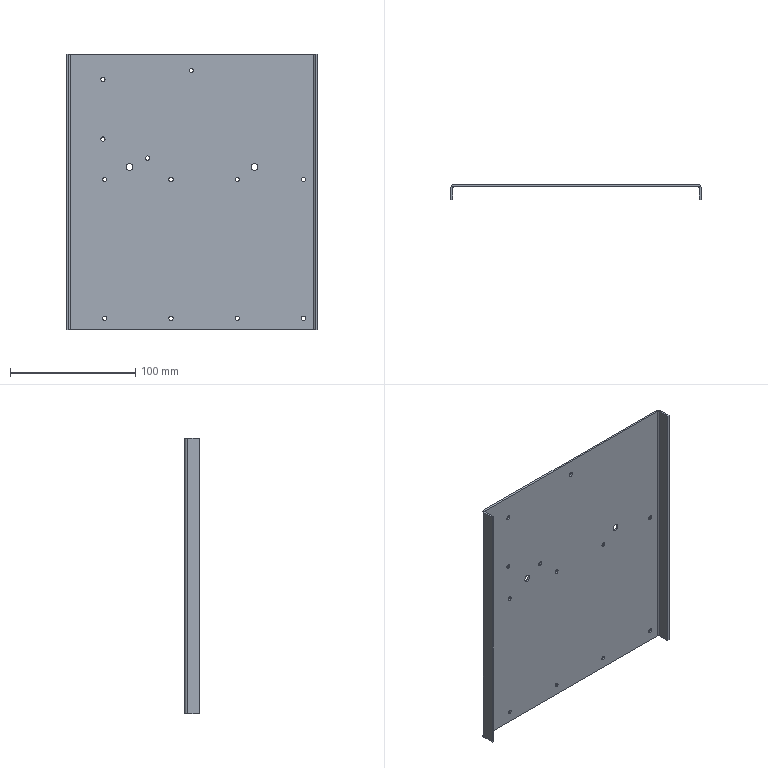Part | NX | features BREP 1 | 1 solid | 28 faces | box 200 x 12 x 220 mm | volume 72200 mm3 | cylinder 18 | plane 10 | commonest cylinder face diameters 3.4 x12 2 x2 5 x2 5.5 x2
STEP:
#1=CARTESIAN_POINT('',(34.5,12.,10.));
#2=VERTEX_POINT('',#1);
#3=CARTESIAN_POINT('',(36.2,12.,10.));
#4=DIRECTION('',(0.,1.,0.));
#5=DIRECTION('',(-1.,0.,0.));
#6=AXIS2_PLACEMENT_3D('',#3,#4,#5);
#7=CIRCLE('',#6,1.7);
#8=EDGE_CURVE('',#2,#2,#7,.T.);
#9=ORIENTED_EDGE('',*,*,#8,.T.);
#10=EDGE_LOOP('',(#9));
#11=FACE_BOUND('',#10,.T.);
#12=CARTESIAN_POINT('',(34.5,10.5,10.));
#13=VERTEX_POINT('',#12);
#14=CARTESIAN_POINT('',(36.2,10.5,10.));
#15=DIRECTION('',(0.,1.,0.));
#16=DIRECTION('',(-1.,0.,0.));
#17=AXIS2_PLACEMENT_3D('',#14,#15,#16);
#18=CIRCLE('',#17,1.7);
#19=EDGE_CURVE('',#13,#13,#18,.T.);
#20=ORIENTED_EDGE('',*,*,#19,.F.);
#21=EDGE_LOOP('',(#20));
#22=FACE_BOUND('',#21,.T.);
#23=CARTESIAN_POINT('',(36.2,2.,10.));
#24=DIRECTION('',(0.,1.,0.));
#25=DIRECTION('',(-1.,0.,0.));
#26=AXIS2_PLACEMENT_3D('',#23,#24,#25);
#27=CYLINDRICAL_SURFACE('',#26,1.7);
#28=ADVANCED_FACE('',(#11,#22),#27,.F.);
#29=CARTESIAN_POINT('',(34.5,12.,-101.));
#30=VERTEX_POINT('',#29);
#31=CARTESIAN_POINT('',(36.2,12.,-101.));
#32=DIRECTION('',(0.,1.,0.));
#33=DIRECTION('',(-1.,0.,0.));
#34=AXIS2_PLACEMENT_3D('',#31,#32,#33);
#35=CIRCLE('',#34,1.7);
#36=EDGE_CURVE('',#30,#30,#35,.T.);
#37=ORIENTED_EDGE('',*,*,#36,.T.);
#38=EDGE_LOOP('',(#37));
#39=FACE_BOUND('',#38,.T.);
#40=CARTESIAN_POINT('',(34.5,10.5,-101.));
#41=VERTEX_POINT('',#40);
#42=CARTESIAN_POINT('',(36.2,10.5,-101.));
#43=DIRECTION('',(0.,1.,0.));
#44=DIRECTION('',(-1.,0.,0.));
#45=AXIS2_PLACEMENT_3D('',#42,#43,#44);
#46=CIRCLE('',#45,1.7);
#47=EDGE_CURVE('',#41,#41,#46,.T.);
#48=ORIENTED_EDGE('',*,*,#47,.F.);
#49=EDGE_LOOP('',(#48));
#50=FACE_BOUND('',#49,.T.);
#51=CARTESIAN_POINT('',(36.2,2.,-101.));
#52=DIRECTION('',(0.,1.,0.));
#53=DIRECTION('',(-1.,0.,0.));
#54=AXIS2_PLACEMENT_3D('',#51,#52,#53);
#55=CYLINDRICAL_SURFACE('',#54,1.7);
#56=ADVANCED_FACE('',(#39,#50),#55,.F.);
#57=CARTESIAN_POINT('',(-72.95,12.,42.321));
#58=VERTEX_POINT('',#57);
#59=CARTESIAN_POINT('',(-71.25,12.,42.321));
#60=DIRECTION('',(0.,1.,0.));
#61=DIRECTION('',(-1.,0.,0.));
#62=AXIS2_PLACEMENT_3D('',#59,#60,#61);
#63=CIRCLE('',#62,1.7);
#64=EDGE_CURVE('',#58,#58,#63,.T.);
#65=ORIENTED_EDGE('',*,*,#64,.T.);
#66=EDGE_LOOP('',(#65));
#67=FACE_BOUND('',#66,.T.);
#68=CARTESIAN_POINT('',(-72.95,10.5,42.321));
#69=VERTEX_POINT('',#68);
#70=CARTESIAN_POINT('',(-71.25,10.5,42.321));
#71=DIRECTION('',(0.,1.,0.));
#72=DIRECTION('',(-1.,0.,0.));
#73=AXIS2_PLACEMENT_3D('',#70,#71,#72);
#74=CIRCLE('',#73,1.7);
#75=EDGE_CURVE('',#69,#69,#74,.T.);
#76=ORIENTED_EDGE('',*,*,#75,.F.);
#77=EDGE_LOOP('',(#76));
#78=FACE_BOUND('',#77,.T.);
#79=CARTESIAN_POINT('',(-71.25,2.,42.321));
#80=DIRECTION('',(0.,1.,0.));
#81=DIRECTION('',(-1.,0.,0.));
#82=AXIS2_PLACEMENT_3D('',#79,#80,#81);
#83=CYLINDRICAL_SURFACE('',#82,1.7);
#84=ADVANCED_FACE('',(#67,#78),#83,.F.);
#85=CARTESIAN_POINT('',(-37.2,12.,27.146));
#86=VERTEX_POINT('',#85);
#87=CARTESIAN_POINT('',(-35.5,12.,27.146));
#88=DIRECTION('',(0.,1.,0.));
#89=DIRECTION('',(-1.,0.,0.));
#90=AXIS2_PLACEMENT_3D('',#87,#88,#89);
#91=CIRCLE('',#90,1.7);
#92=EDGE_CURVE('',#86,#86,#91,.T.);
#93=ORIENTED_EDGE('',*,*,#92,.T.);
#94=EDGE_LOOP('',(#93));
#95=FACE_BOUND('',#94,.T.);
#96=CARTESIAN_POINT('',(-37.2,10.5,27.146));
#97=VERTEX_POINT('',#96);
#98=CARTESIAN_POINT('',(-35.5,10.5,27.146));
#99=DIRECTION('',(0.,1.,0.));
#100=DIRECTION('',(-1.,0.,0.));
#101=AXIS2_PLACEMENT_3D('',#98,#99,#100);
#102=CIRCLE('',#101,1.7);
#103=EDGE_CURVE('',#97,#97,#102,.T.);
#104=ORIENTED_EDGE('',*,*,#103,.F.);
#105=EDGE_LOOP('',(#104));
#106=FACE_BOUND('',#105,.T.);
#107=CARTESIAN_POINT('',(-35.5,2.,27.146));
#108=DIRECTION('',(0.,1.,0.));
#109=DIRECTION('',(-1.,0.,0.));
#110=AXIS2_PLACEMENT_3D('',#107,#108,#109);
#111=CYLINDRICAL_SURFACE('',#110,1.7);
#112=ADVANCED_FACE('',(#95,#106),#111,.F.);
#113=CARTESIAN_POINT('',(-2.2,12.,97.146));
#114=VERTEX_POINT('',#113);
#115=CARTESIAN_POINT('',(-0.5,12.,97.146));
#116=DIRECTION('',(0.,1.,0.));
#117=DIRECTION('',(-1.,0.,0.));
#118=AXIS2_PLACEMENT_3D('',#115,#116,#117);
#119=CIRCLE('',#118,1.7);
#120=EDGE_CURVE('',#114,#114,#119,.T.);
#121=ORIENTED_EDGE('',*,*,#120,.T.);
#122=EDGE_LOOP('',(#121));
#123=FACE_BOUND('',#122,.T.);
#124=CARTESIAN_POINT('',(-2.2,10.5,97.146));
#125=VERTEX_POINT('',#124);
#126=CARTESIAN_POINT('',(-0.5,10.5,97.146));
#127=DIRECTION('',(0.,1.,0.));
#128=DIRECTION('',(-1.,0.,0.));
#129=AXIS2_PLACEMENT_3D('',#126,#127,#128);
#130=CIRCLE('',#129,1.7);
#131=EDGE_CURVE('',#125,#125,#130,.T.);
#132=ORIENTED_EDGE('',*,*,#131,.F.);
#133=EDGE_LOOP('',(#132));
#134=FACE_BOUND('',#133,.T.);
#135=CARTESIAN_POINT('',(-0.5,2.,97.146));
#136=DIRECTION('',(0.,1.,0.));
#137=DIRECTION('',(-1.,0.,0.));
#138=AXIS2_PLACEMENT_3D('',#135,#136,#137);
#139=CYLINDRICAL_SURFACE('',#138,1.7);
#140=ADVANCED_FACE('',(#123,#134),#139,.F.);
#141=CARTESIAN_POINT('',(-72.95,12.,90.071));
#142=VERTEX_POINT('',#141);
#143=CARTESIAN_POINT('',(-71.25,12.,90.071));
#144=DIRECTION('',(0.,1.,0.));
#145=DIRECTION('',(-1.,0.,0.));
#146=AXIS2_PLACEMENT_3D('',#143,#144,#145);
#147=CIRCLE('',#146,1.7);
#148=EDGE_CURVE('',#142,#142,#147,.T.);
#149=ORIENTED_EDGE('',*,*,#148,.T.);
#150=EDGE_LOOP('',(#149));
#151=FACE_BOUND('',#150,.T.);
#152=CARTESIAN_POINT('',(-72.95,10.5,90.071));
#153=VERTEX_POINT('',#152);
#154=CARTESIAN_POINT('',(-71.25,10.5,90.071));
#155=DIRECTION('',(0.,1.,0.));
#156=DIRECTION('',(-1.,0.,0.));
#157=AXIS2_PLACEMENT_3D('',#154,#155,#156);
#158=CIRCLE('',#157,1.7);
#159=EDGE_CURVE('',#153,#153,#158,.T.);
#160=ORIENTED_EDGE('',*,*,#159,.F.);
#161=EDGE_LOOP('',(#160));
#162=FACE_BOUND('',#161,.T.);
#163=CARTESIAN_POINT('',(-71.25,2.,90.071));
#164=DIRECTION('',(0.,1.,0.));
#165=DIRECTION('',(-1.,0.,0.));
#166=AXIS2_PLACEMENT_3D('',#163,#164,#165);
#167=CYLINDRICAL_SURFACE('',#166,1.7);
#168=ADVANCED_FACE('',(#151,#162),#167,.F.);
#169=CARTESIAN_POINT('',(87.5,12.,-101.));
#170=VERTEX_POINT('',#169);
#171=CARTESIAN_POINT('',(89.2,12.,-101.));
#172=DIRECTION('',(0.,1.,0.));
#173=DIRECTION('',(-1.,0.,0.));
#174=AXIS2_PLACEMENT_3D('',#171,#172,#173);
#175=CIRCLE('',#174,1.7);
#176=EDGE_CURVE('',#170,#170,#175,.T.);
#177=ORIENTED_EDGE('',*,*,#176,.T.);
#178=EDGE_LOOP('',(#177));
#179=FACE_BOUND('',#178,.T.);
#180=CARTESIAN_POINT('',(87.5,10.5,-101.));
#181=VERTEX_POINT('',#180);
#182=CARTESIAN_POINT('',(89.2,10.5,-101.));
#183=DIRECTION('',(0.,1.,0.));
#184=DIRECTION('',(-1.,0.,0.));
#185=AXIS2_PLACEMENT_3D('',#182,#183,#184);
#186=CIRCLE('',#185,1.7);
#187=EDGE_CURVE('',#181,#181,#186,.T.);
#188=ORIENTED_EDGE('',*,*,#187,.F.);
#189=EDGE_LOOP('',(#188));
#190=FACE_BOUND('',#189,.T.);
#191=CARTESIAN_POINT('',(89.2,2.,-101.));
#192=DIRECTION('',(0.,1.,0.));
#193=DIRECTION('',(-1.,0.,0.));
#194=AXIS2_PLACEMENT_3D('',#191,#192,#193);
#195=CYLINDRICAL_SURFACE('',#194,1.7);
#196=ADVANCED_FACE('',(#179,#190),#195,.F.);
#197=CARTESIAN_POINT('',(87.5,12.,10.));
#198=VERTEX_POINT('',#197);
#199=CARTESIAN_POINT('',(89.2,12.,10.));
#200=DIRECTION('',(0.,1.,0.));
#201=DIRECTION('',(-1.,0.,0.));
#202=AXIS2_PLACEMENT_3D('',#199,#200,#201);
#203=CIRCLE('',#202,1.7);
#204=EDGE_CURVE('',#198,#198,#203,.T.);
#205=ORIENTED_EDGE('',*,*,#204,.T.);
#206=EDGE_LOOP('',(#205));
#207=FACE_BOUND('',#206,.T.);
#208=CARTESIAN_POINT('',(87.5,10.5,10.));
#209=VERTEX_POINT('',#208);
#210=CARTESIAN_POINT('',(89.2,10.5,10.));
#211=DIRECTION('',(0.,1.,0.));
#212=DIRECTION('',(-1.,0.,0.));
#213=AXIS2_PLACEMENT_3D('',#210,#211,#212);
#214=CIRCLE('',#213,1.7);
#215=EDGE_CURVE('',#209,#209,#214,.T.);
#216=ORIENTED_EDGE('',*,*,#215,.F.);
#217=EDGE_LOOP('',(#216));
#218=FACE_BOUND('',#217,.T.);
#219=CARTESIAN_POINT('',(89.2,2.,10.));
#220=DIRECTION('',(0.,1.,0.));
#221=DIRECTION('',(-1.,0.,0.));
#222=AXIS2_PLACEMENT_3D('',#219,#220,#221);
#223=CYLINDRICAL_SURFACE('',#222,1.7);
#224=ADVANCED_FACE('',(#207,#218),#223,.F.);
#225=CARTESIAN_POINT('',(52.75,12.,20.));
#226=VERTEX_POINT('',#225);
#227=CARTESIAN_POINT('',(50.,12.,20.));
#228=DIRECTION('',(0.,1.,0.));
#229=DIRECTION('',(1.,0.,0.));
#230=AXIS2_PLACEMENT_3D('',#227,#228,#229);
#231=CIRCLE('',#230,2.75);
#232=EDGE_CURVE('',#226,#226,#231,.T.);
#233=ORIENTED_EDGE('',*,*,#232,.T.);
#234=EDGE_LOOP('',(#233));
#235=FACE_BOUND('',#234,.T.);
#236=CARTESIAN_POINT('',(47.25,10.5,20.));
#237=VERTEX_POINT('',#236);
#238=CARTESIAN_POINT('',(50.,10.5,20.));
#239=DIRECTION('',(0.,1.,0.));
#240=DIRECTION('',(-1.,0.,0.));
#241=AXIS2_PLACEMENT_3D('',#238,#239,#240);
#242=CIRCLE('',#241,2.75);
#243=EDGE_CURVE('',#237,#237,#242,.T.);
#244=ORIENTED_EDGE('',*,*,#243,.F.);
#245=EDGE_LOOP('',(#244));
#246=FACE_BOUND('',#245,.T.);
#247=CARTESIAN_POINT('',(50.,2.,20.));
#248=DIRECTION('',(0.,1.,0.));
#249=DIRECTION('',(-1.,0.,0.));
#250=AXIS2_PLACEMENT_3D('',#247,#248,#249);
#251=CYLINDRICAL_SURFACE('',#250,2.75);
#252=ADVANCED_FACE('',(#235,#246),#251,.F.);
#253=CARTESIAN_POINT('',(-52.75,12.,20.));
#254=VERTEX_POINT('',#253);
#255=CARTESIAN_POINT('',(-50.,12.,20.));
#256=DIRECTION('',(0.,1.,0.));
#257=DIRECTION('',(-1.,0.,0.));
#258=AXIS2_PLACEMENT_3D('',#255,#256,#257);
#259=CIRCLE('',#258,2.75);
#260=EDGE_CURVE('',#254,#254,#259,.T.);
#261=ORIENTED_EDGE('',*,*,#260,.T.);
#262=EDGE_LOOP('',(#261));
#263=FACE_BOUND('',#262,.T.);
#264=CARTESIAN_POINT('',(-52.75,10.5,20.));
#265=VERTEX_POINT('',#264);
#266=CARTESIAN_POINT('',(-50.,10.5,20.));
#267=DIRECTION('',(0.,1.,0.));
#268=DIRECTION('',(-1.,0.,0.));
#269=AXIS2_PLACEMENT_3D('',#266,#267,#268);
#270=CIRCLE('',#269,2.75);
#271=EDGE_CURVE('',#265,#265,#270,.T.);
#272=ORIENTED_EDGE('',*,*,#271,.F.);
#273=EDGE_LOOP('',(#272));
#274=FACE_BOUND('',#273,.T.);
#275=CARTESIAN_POINT('',(-50.,2.,20.));
#276=DIRECTION('',(0.,1.,0.));
#277=DIRECTION('',(-1.,0.,0.));
#278=AXIS2_PLACEMENT_3D('',#275,#276,#277);
#279=CYLINDRICAL_SURFACE('',#278,2.75);
#280=ADVANCED_FACE('',(#263,#274),#279,.F.);
#281=CARTESIAN_POINT('',(-18.5,12.,-101.));
#282=VERTEX_POINT('',#281);
#283=CARTESIAN_POINT('',(-16.8,12.,-101.));
#284=DIRECTION('',(0.,1.,0.));
#285=DIRECTION('',(-1.,0.,0.));
#286=AXIS2_PLACEMENT_3D('',#283,#284,#285);
#287=CIRCLE('',#286,1.7);
#288=EDGE_CURVE('',#282,#282,#287,.T.);
#289=ORIENTED_EDGE('',*,*,#288,.T.);
#290=EDGE_LOOP('',(#289));
#291=FACE_BOUND('',#290,.T.);
#292=CARTESIAN_POINT('',(-18.5,10.5,-101.));
#293=VERTEX_POINT('',#292);
#294=CARTESIAN_POINT('',(-16.8,10.5,-101.));
#295=DIRECTION('',(0.,1.,0.));
#296=DIRECTION('',(-1.,0.,0.));
#297=AXIS2_PLACEMENT_3D('',#294,#295,#296);
#298=CIRCLE('',#297,1.7);
#299=EDGE_CURVE('',#293,#293,#298,.T.);
#300=ORIENTED_EDGE('',*,*,#299,.F.);
#301=EDGE_LOOP('',(#300));
#302=FACE_BOUND('',#301,.T.);
#303=CARTESIAN_POINT('',(-16.8,2.,-101.));
#304=DIRECTION('',(0.,1.,0.));
#305=DIRECTION('',(-1.,0.,0.));
#306=AXIS2_PLACEMENT_3D('',#303,#304,#305);
#307=CYLINDRICAL_SURFACE('',#306,1.7);
#308=ADVANCED_FACE('',(#291,#302),#307,.F.);
#309=CARTESIAN_POINT('',(-71.5,12.,-101.));
#310=VERTEX_POINT('',#309);
#311=CARTESIAN_POINT('',(-69.8,12.,-101.));
#312=DIRECTION('',(0.,1.,0.));
#313=DIRECTION('',(-1.,0.,0.));
#314=AXIS2_PLACEMENT_3D('',#311,#312,#313);
#315=CIRCLE('',#314,1.7);
#316=EDGE_CURVE('',#310,#310,#315,.T.);
#317=ORIENTED_EDGE('',*,*,#316,.T.);
#318=EDGE_LOOP('',(#317));
#319=FACE_BOUND('',#318,.T.);
#320=CARTESIAN_POINT('',(-71.5,10.5,-101.));
#321=VERTEX_POINT('',#320);
#322=CARTESIAN_POINT('',(-69.8,10.5,-101.));
#323=DIRECTION('',(0.,1.,0.));
#324=DIRECTION('',(-1.,0.,0.));
#325=AXIS2_PLACEMENT_3D('',#322,#323,#324);
#326=CIRCLE('',#325,1.7);
#327=EDGE_CURVE('',#321,#321,#326,.T.);
#328=ORIENTED_EDGE('',*,*,#327,.F.);
#329=EDGE_LOOP('',(#328));
#330=FACE_BOUND('',#329,.T.);
#331=CARTESIAN_POINT('',(-69.8,2.,-101.));
#332=DIRECTION('',(0.,1.,0.));
#333=DIRECTION('',(-1.,0.,0.));
#334=AXIS2_PLACEMENT_3D('',#331,#332,#333);
#335=CYLINDRICAL_SURFACE('',#334,1.7);
#336=ADVANCED_FACE('',(#319,#330),#335,.F.);
#337=CARTESIAN_POINT('',(-18.5,12.,10.));
#338=VERTEX_POINT('',#337);
#339=CARTESIAN_POINT('',(-16.8,12.,10.));
#340=DIRECTION('',(0.,1.,0.));
#341=DIRECTION('',(-1.,0.,0.));
#342=AXIS2_PLACEMENT_3D('',#339,#340,#341);
#343=CIRCLE('',#342,1.7);
#344=EDGE_CURVE('',#338,#338,#343,.T.);
#345=ORIENTED_EDGE('',*,*,#344,.T.);
#346=EDGE_LOOP('',(#345));
#347=FACE_BOUND('',#346,.T.);
#348=CARTESIAN_POINT('',(-18.5,10.5,10.));
#349=VERTEX_POINT('',#348);
#350=CARTESIAN_POINT('',(-16.8,10.5,10.));
#351=DIRECTION('',(0.,1.,0.));
#352=DIRECTION('',(-1.,0.,0.));
#353=AXIS2_PLACEMENT_3D('',#350,#351,#352);
#354=CIRCLE('',#353,1.7);
#355=EDGE_CURVE('',#349,#349,#354,.T.);
#356=ORIENTED_EDGE('',*,*,#355,.F.);
#357=EDGE_LOOP('',(#356));
#358=FACE_BOUND('',#357,.T.);
#359=CARTESIAN_POINT('',(-16.8,2.,10.));
#360=DIRECTION('',(0.,1.,0.));
#361=DIRECTION('',(-1.,0.,0.));
#362=AXIS2_PLACEMENT_3D('',#359,#360,#361);
#363=CYLINDRICAL_SURFACE('',#362,1.7);
#364=ADVANCED_FACE('',(#347,#358),#363,.F.);
#365=CARTESIAN_POINT('',(-71.5,12.,10.));
#366=VERTEX_POINT('',#365);
#367=CARTESIAN_POINT('',(-69.8,12.,10.));
#368=DIRECTION('',(0.,1.,0.));
#369=DIRECTION('',(-1.,0.,0.));
#370=AXIS2_PLACEMENT_3D('',#367,#368,#369);
#371=CIRCLE('',#370,1.7);
#372=EDGE_CURVE('',#366,#366,#371,.T.);
#373=ORIENTED_EDGE('',*,*,#372,.T.);
#374=EDGE_LOOP('',(#373));
#375=FACE_BOUND('',#374,.T.);
#376=CARTESIAN_POINT('',(-71.5,10.5,10.));
#377=VERTEX_POINT('',#376);
#378=CARTESIAN_POINT('',(-69.8,10.5,10.));
#379=DIRECTION('',(0.,1.,0.));
#380=DIRECTION('',(-1.,0.,0.));
#381=AXIS2_PLACEMENT_3D('',#378,#379,#380);
#382=CIRCLE('',#381,1.7);
#383=EDGE_CURVE('',#377,#377,#382,.T.);
#384=ORIENTED_EDGE('',*,*,#383,.F.);
#385=EDGE_LOOP('',(#384));
#386=FACE_BOUND('',#385,.T.);
#387=CARTESIAN_POINT('',(-69.8,2.,10.));
#388=DIRECTION('',(0.,1.,0.));
#389=DIRECTION('',(-1.,0.,0.));
#390=AXIS2_PLACEMENT_3D('',#387,#388,#389);
#391=CYLINDRICAL_SURFACE('',#390,1.7);
#392=ADVANCED_FACE('',(#375,#386),#391,.F.);
#393=CARTESIAN_POINT('',(-98.5,9.5,110.));
#394=VERTEX_POINT('',#393);
#395=CARTESIAN_POINT('',(-97.5,10.5,110.));
#396=VERTEX_POINT('',#395);
#397=CARTESIAN_POINT('',(-97.5,9.5,110.));
#398=DIRECTION('',(0.,0.,-1.));
#399=DIRECTION('',(1.,0.,0.));
#400=AXIS2_PLACEMENT_3D('',#397,#398,#399);
#401=CIRCLE('',#400,1.);
#402=EDGE_CURVE('',#394,#396,#401,.T.);
#403=ORIENTED_EDGE('',*,*,#402,.T.);
#404=CARTESIAN_POINT('',(97.5,10.5,110.));
#405=VERTEX_POINT('',#404);
#406=CARTESIAN_POINT('',(-100.,10.5,110.));
#407=DIRECTION('',(1.,0.,0.));
#408=VECTOR('',#407,1000.);
#409=LINE('',#406,#408);
#410=EDGE_CURVE('',#396,#405,#409,.T.);
#411=ORIENTED_EDGE('',*,*,#410,.T.);
#412=CARTESIAN_POINT('',(98.5,9.5,110.));
#413=VERTEX_POINT('',#412);
#414=CARTESIAN_POINT('',(97.5,9.5,110.));
#415=DIRECTION('',(0.,0.,-1.));
#416=DIRECTION('',(1.,0.,0.));
#417=AXIS2_PLACEMENT_3D('',#414,#415,#416);
#418=CIRCLE('',#417,1.);
#419=EDGE_CURVE('',#405,#413,#418,.T.);
#420=ORIENTED_EDGE('',*,*,#419,.T.);
#421=CARTESIAN_POINT('',(98.5,0.,110.));
#422=VERTEX_POINT('',#421);
#423=CARTESIAN_POINT('',(98.5,12.,110.));
#424=DIRECTION('',(0.,-1.,0.));
#425=VECTOR('',#424,1000.);
#426=LINE('',#423,#425);
#427=EDGE_CURVE('',#413,#422,#426,.T.);
#428=ORIENTED_EDGE('',*,*,#427,.T.);
#429=CARTESIAN_POINT('',(100.,0.,110.));
#430=VERTEX_POINT('',#429);
#431=CARTESIAN_POINT('',(100.,0.,110.));
#432=DIRECTION('',(-1.,0.,0.));
#433=VECTOR('',#432,1000.);
#434=LINE('',#431,#433);
#435=EDGE_CURVE('',#430,#422,#434,.T.);
#436=ORIENTED_EDGE('',*,*,#435,.F.);
#437=CARTESIAN_POINT('',(100.,9.5,110.));
#438=VERTEX_POINT('',#437);
#439=CARTESIAN_POINT('',(100.,12.,110.));
#440=DIRECTION('',(0.,-1.,0.));
#441=VECTOR('',#440,1000.);
#442=LINE('',#439,#441);
#443=EDGE_CURVE('',#438,#430,#442,.T.);
#444=ORIENTED_EDGE('',*,*,#443,.F.);
#445=CARTESIAN_POINT('',(97.5,12.,110.));
#446=VERTEX_POINT('',#445);
#447=CARTESIAN_POINT('',(97.5,9.5,110.));
#448=DIRECTION('',(0.,0.,-1.));
#449=DIRECTION('',(1.,0.,0.));
#450=AXIS2_PLACEMENT_3D('',#447,#448,#449);
#451=CIRCLE('',#450,2.5);
#452=EDGE_CURVE('',#446,#438,#451,.T.);
#453=ORIENTED_EDGE('',*,*,#452,.F.);
#454=CARTESIAN_POINT('',(-97.5,12.,110.));
#455=VERTEX_POINT('',#454);
#456=CARTESIAN_POINT('',(-100.,12.,110.));
#457=DIRECTION('',(1.,0.,0.));
#458=VECTOR('',#457,1000.);
#459=LINE('',#456,#458);
#460=EDGE_CURVE('',#455,#446,#459,.T.);
#461=ORIENTED_EDGE('',*,*,#460,.F.);
#462=CARTESIAN_POINT('',(-100.,9.5,110.));
#463=VERTEX_POINT('',#462);
#464=CARTESIAN_POINT('',(-97.5,9.5,110.));
#465=DIRECTION('',(0.,0.,-1.));
#466=DIRECTION('',(1.,0.,0.));
#467=AXIS2_PLACEMENT_3D('',#464,#465,#466);
#468=CIRCLE('',#467,2.5);
#469=EDGE_CURVE('',#463,#455,#468,.T.);
#470=ORIENTED_EDGE('',*,*,#469,.F.);
#471=CARTESIAN_POINT('',(-100.,0.,110.));
#472=VERTEX_POINT('',#471);
#473=CARTESIAN_POINT('',(-100.,0.,110.));
#474=DIRECTION('',(0.,1.,0.));
#475=VECTOR('',#474,1000.);
#476=LINE('',#473,#475);
#477=EDGE_CURVE('',#472,#463,#476,.T.);
#478=ORIENTED_EDGE('',*,*,#477,.F.);
#479=CARTESIAN_POINT('',(-98.5,0.,110.));
#480=VERTEX_POINT('',#479);
#481=CARTESIAN_POINT('',(-98.5,0.,110.));
#482=DIRECTION('',(-1.,0.,0.));
#483=VECTOR('',#482,1000.);
#484=LINE('',#481,#483);
#485=EDGE_CURVE('',#480,#472,#484,.T.);
#486=ORIENTED_EDGE('',*,*,#485,.F.);
#487=CARTESIAN_POINT('',(-98.5,0.,110.));
#488=DIRECTION('',(0.,1.,0.));
#489=VECTOR('',#488,1000.);
#490=LINE('',#487,#489);
#491=EDGE_CURVE('',#480,#394,#490,.T.);
#492=ORIENTED_EDGE('',*,*,#491,.T.);
#493=EDGE_LOOP('',(#403,#411,#420,#428,#436,#444,#453,#461,#470,#478,#486,#492));
#494=FACE_BOUND('',#493,.T.);
#495=CARTESIAN_POINT('',(-97.5,12.,110.));
#496=DIRECTION('',(0.,0.,1.));
#497=DIRECTION('',(1.,0.,0.));
#498=AXIS2_PLACEMENT_3D('',#495,#496,#497);
#499=PLANE('',#498);
#500=ADVANCED_FACE('',(#494),#499,.T.);
#501=CARTESIAN_POINT('',(-98.5,9.5,-110.));
#502=VERTEX_POINT('',#501);
#503=CARTESIAN_POINT('',(-97.5,10.5,-110.));
#504=VERTEX_POINT('',#503);
#505=CARTESIAN_POINT('',(-97.5,9.5,-110.));
#506=DIRECTION('',(0.,0.,-1.));
#507=DIRECTION('',(1.,0.,0.));
#508=AXIS2_PLACEMENT_3D('',#505,#506,#507);
#509=CIRCLE('',#508,1.);
#510=EDGE_CURVE('',#502,#504,#509,.T.);
#511=ORIENTED_EDGE('',*,*,#510,.F.);
#512=CARTESIAN_POINT('',(-98.5,0.,-110.));
#513=VERTEX_POINT('',#512);
#514=CARTESIAN_POINT('',(-98.5,0.,-110.));
#515=DIRECTION('',(0.,1.,0.));
#516=VECTOR('',#515,1000.);
#517=LINE('',#514,#516);
#518=EDGE_CURVE('',#513,#502,#517,.T.);
#519=ORIENTED_EDGE('',*,*,#518,.F.);
#520=CARTESIAN_POINT('',(-100.,0.,-110.));
#521=VERTEX_POINT('',#520);
#522=CARTESIAN_POINT('',(-98.5,0.,-110.));
#523=DIRECTION('',(-1.,0.,0.));
#524=VECTOR('',#523,1000.);
#525=LINE('',#522,#524);
#526=EDGE_CURVE('',#513,#521,#525,.T.);
#527=ORIENTED_EDGE('',*,*,#526,.T.);
#528=CARTESIAN_POINT('',(-100.,9.5,-110.));
#529=VERTEX_POINT('',#528);
#530=CARTESIAN_POINT('',(-100.,0.,-110.));
#531=DIRECTION('',(0.,1.,0.));
#532=VECTOR('',#531,1000.);
#533=LINE('',#530,#532);
#534=EDGE_CURVE('',#521,#529,#533,.T.);
#535=ORIENTED_EDGE('',*,*,#534,.T.);
#536=CARTESIAN_POINT('',(-97.5,12.,-110.));
#537=VERTEX_POINT('',#536);
#538=CARTESIAN_POINT('',(-97.5,9.5,-110.));
#539=DIRECTION('',(0.,0.,-1.));
#540=DIRECTION('',(1.,0.,0.));
#541=AXIS2_PLACEMENT_3D('',#538,#539,#540);
#542=CIRCLE('',#541,2.5);
#543=EDGE_CURVE('',#529,#537,#542,.T.);
#544=ORIENTED_EDGE('',*,*,#543,.T.);
#545=CARTESIAN_POINT('',(97.5,12.,-110.));
#546=VERTEX_POINT('',#545);
#547=CARTESIAN_POINT('',(-100.,12.,-110.));
#548=DIRECTION('',(1.,0.,0.));
#549=VECTOR('',#548,1000.);
#550=LINE('',#547,#549);
#551=EDGE_CURVE('',#537,#546,#550,.T.);
#552=ORIENTED_EDGE('',*,*,#551,.T.);
#553=CARTESIAN_POINT('',(100.,9.5,-110.));
#554=VERTEX_POINT('',#553);
#555=CARTESIAN_POINT('',(97.5,9.5,-110.));
#556=DIRECTION('',(0.,0.,-1.));
#557=DIRECTION('',(1.,0.,0.));
#558=AXIS2_PLACEMENT_3D('',#555,#556,#557);
#559=CIRCLE('',#558,2.5);
#560=EDGE_CURVE('',#546,#554,#559,.T.);
#561=ORIENTED_EDGE('',*,*,#560,.T.);
#562=CARTESIAN_POINT('',(100.,0.,-110.));
#563=VERTEX_POINT('',#562);
#564=CARTESIAN_POINT('',(100.,12.,-110.));
#565=DIRECTION('',(0.,-1.,0.));
#566=VECTOR('',#565,1000.);
#567=LINE('',#564,#566);
#568=EDGE_CURVE('',#554,#563,#567,.T.);
#569=ORIENTED_EDGE('',*,*,#568,.T.);
#570=CARTESIAN_POINT('',(98.5,0.,-110.));
#571=VERTEX_POINT('',#570);
#572=CARTESIAN_POINT('',(100.,0.,-110.));
#573=DIRECTION('',(-1.,0.,0.));
#574=VECTOR('',#573,1000.);
#575=LINE('',#572,#574);
#576=EDGE_CURVE('',#563,#571,#575,.T.);
#577=ORIENTED_EDGE('',*,*,#576,.T.);
#578=CARTESIAN_POINT('',(98.5,9.5,-110.));
#579=VERTEX_POINT('',#578);
#580=CARTESIAN_POINT('',(98.5,12.,-110.));
#581=DIRECTION('',(0.,-1.,0.));
#582=VECTOR('',#581,1000.);
#583=LINE('',#580,#582);
#584=EDGE_CURVE('',#579,#571,#583,.T.);
#585=ORIENTED_EDGE('',*,*,#584,.F.);
#586=CARTESIAN_POINT('',(97.5,10.5,-110.));
#587=VERTEX_POINT('',#586);
#588=CARTESIAN_POINT('',(97.5,9.5,-110.));
#589=DIRECTION('',(0.,0.,-1.));
#590=DIRECTION('',(1.,0.,0.));
#591=AXIS2_PLACEMENT_3D('',#588,#589,#590);
#592=CIRCLE('',#591,1.);
#593=EDGE_CURVE('',#587,#579,#592,.T.);
#594=ORIENTED_EDGE('',*,*,#593,.F.);
#595=CARTESIAN_POINT('',(-100.,10.5,-110.));
#596=DIRECTION('',(1.,0.,0.));
#597=VECTOR('',#596,1000.);
#598=LINE('',#595,#597);
#599=EDGE_CURVE('',#504,#587,#598,.T.);
#600=ORIENTED_EDGE('',*,*,#599,.F.);
#601=EDGE_LOOP('',(#511,#519,#527,#535,#544,#552,#561,#569,#577,#585,#594,#600));
#602=FACE_BOUND('',#601,.T.);
#603=CARTESIAN_POINT('',(-100.,9.5,-110.));
#604=DIRECTION('',(0.,0.,-1.));
#605=DIRECTION('',(-1.,0.,0.));
#606=AXIS2_PLACEMENT_3D('',#603,#604,#605);
#607=PLANE('',#606);
#608=ADVANCED_FACE('',(#602),#607,.T.);
#609=ORIENTED_EDGE('',*,*,#584,.T.);
#610=CARTESIAN_POINT('',(98.5,0.,110.));
#611=DIRECTION('',(0.,0.,-1.));
#612=VECTOR('',#611,1000.);
#613=LINE('',#610,#612);
#614=EDGE_CURVE('',#422,#571,#613,.T.);
#615=ORIENTED_EDGE('',*,*,#614,.F.);
#616=ORIENTED_EDGE('',*,*,#427,.F.);
#617=CARTESIAN_POINT('',(98.5,9.5,110.));
#618=DIRECTION('',(0.,0.,-1.));
#619=VECTOR('',#618,1000.);
#620=LINE('',#617,#619);
#621=EDGE_CURVE('',#413,#579,#620,.T.);
#622=ORIENTED_EDGE('',*,*,#621,.T.);
#623=EDGE_LOOP('',(#609,#615,#616,#622));
#624=FACE_BOUND('',#623,.T.);
#625=CARTESIAN_POINT('',(98.5,12.,110.));
#626=DIRECTION('',(1.,0.,0.));
#627=DIRECTION('',(0.,0.,-1.));
#628=AXIS2_PLACEMENT_3D('',#625,#626,#627);
#629=PLANE('',#628);
#630=ADVANCED_FACE('',(#624),#629,.F.);
#631=ORIENTED_EDGE('',*,*,#576,.F.);
#632=CARTESIAN_POINT('',(100.,0.,110.));
#633=DIRECTION('',(0.,0.,-1.));
#634=VECTOR('',#633,1000.);
#635=LINE('',#632,#634);
#636=EDGE_CURVE('',#430,#563,#635,.T.);
#637=ORIENTED_EDGE('',*,*,#636,.F.);
#638=ORIENTED_EDGE('',*,*,#435,.T.);
#639=ORIENTED_EDGE('',*,*,#614,.T.);
#640=EDGE_LOOP('',(#631,#637,#638,#639));
#641=FACE_BOUND('',#640,.T.);
#642=CARTESIAN_POINT('',(100.,0.,110.));
#643=DIRECTION('',(0.,-1.,0.));
#644=DIRECTION('',(1.,0.,0.));
#645=AXIS2_PLACEMENT_3D('',#642,#643,#644);
#646=PLANE('',#645);
#647=ADVANCED_FACE('',(#641),#646,.T.);
#648=ORIENTED_EDGE('',*,*,#568,.F.);
#649=CARTESIAN_POINT('',(100.,9.5,110.));
#650=DIRECTION('',(0.,0.,-1.));
#651=VECTOR('',#650,1000.);
#652=LINE('',#649,#651);
#653=EDGE_CURVE('',#438,#554,#652,.T.);
#654=ORIENTED_EDGE('',*,*,#653,.F.);
#655=ORIENTED_EDGE('',*,*,#443,.T.);
#656=ORIENTED_EDGE('',*,*,#636,.T.);
#657=EDGE_LOOP('',(#648,#654,#655,#656));
#658=FACE_BOUND('',#657,.T.);
#659=CARTESIAN_POINT('',(100.,12.,110.));
#660=DIRECTION('',(1.,0.,0.));
#661=DIRECTION('',(0.,0.,-1.));
#662=AXIS2_PLACEMENT_3D('',#659,#660,#661);
#663=PLANE('',#662);
#664=ADVANCED_FACE('',(#658),#663,.T.);
#665=ORIENTED_EDGE('',*,*,#560,.F.);
#666=CARTESIAN_POINT('',(97.5,12.,110.));
#667=DIRECTION('',(0.,0.,-1.));
#668=VECTOR('',#667,1000.);
#669=LINE('',#666,#668);
#670=EDGE_CURVE('',#446,#546,#669,.T.);
#671=ORIENTED_EDGE('',*,*,#670,.F.);
#672=ORIENTED_EDGE('',*,*,#452,.T.);
#673=ORIENTED_EDGE('',*,*,#653,.T.);
#674=EDGE_LOOP('',(#665,#671,#672,#673));
#675=FACE_BOUND('',#674,.T.);
#676=CARTESIAN_POINT('',(97.5,9.5,110.));
#677=DIRECTION('',(0.,0.,-1.));
#678=DIRECTION('',(-1.,0.,0.));
#679=AXIS2_PLACEMENT_3D('',#676,#677,#678);
#680=CYLINDRICAL_SURFACE('',#679,2.5);
#681=ADVANCED_FACE('',(#675),#680,.T.);
#682=ORIENTED_EDGE('',*,*,#8,.F.);
#683=EDGE_LOOP('',(#682));
#684=FACE_BOUND('',#683,.T.);
#685=ORIENTED_EDGE('',*,*,#36,.F.);
#686=EDGE_LOOP('',(#685));
#687=FACE_BOUND('',#686,.T.);
#688=ORIENTED_EDGE('',*,*,#64,.F.);
#689=EDGE_LOOP('',(#688));
#690=FACE_BOUND('',#689,.T.);
#691=ORIENTED_EDGE('',*,*,#92,.F.);
#692=EDGE_LOOP('',(#691));
#693=FACE_BOUND('',#692,.T.);
#694=ORIENTED_EDGE('',*,*,#120,.F.);
#695=EDGE_LOOP('',(#694));
#696=FACE_BOUND('',#695,.T.);
#697=ORIENTED_EDGE('',*,*,#148,.F.);
#698=EDGE_LOOP('',(#697));
#699=FACE_BOUND('',#698,.T.);
#700=ORIENTED_EDGE('',*,*,#176,.F.);
#701=EDGE_LOOP('',(#700));
#702=FACE_BOUND('',#701,.T.);
#703=ORIENTED_EDGE('',*,*,#204,.F.);
#704=EDGE_LOOP('',(#703));
#705=FACE_BOUND('',#704,.T.);
#706=ORIENTED_EDGE('',*,*,#232,.F.);
#707=EDGE_LOOP('',(#706));
#708=FACE_BOUND('',#707,.T.);
#709=ORIENTED_EDGE('',*,*,#260,.F.);
#710=EDGE_LOOP('',(#709));
#711=FACE_BOUND('',#710,.T.);
#712=ORIENTED_EDGE('',*,*,#551,.F.);
#713=CARTESIAN_POINT('',(-97.5,12.,110.));
#714=DIRECTION('',(0.,0.,-1.));
#715=VECTOR('',#714,1000.);
#716=LINE('',#713,#715);
#717=EDGE_CURVE('',#455,#537,#716,.T.);
#718=ORIENTED_EDGE('',*,*,#717,.F.);
#719=ORIENTED_EDGE('',*,*,#460,.T.);
#720=ORIENTED_EDGE('',*,*,#670,.T.);
#721=EDGE_LOOP('',(#712,#718,#719,#720));
#722=FACE_BOUND('',#721,.T.);
#723=ORIENTED_EDGE('',*,*,#288,.F.);
#724=EDGE_LOOP('',(#723));
#725=FACE_BOUND('',#724,.T.);
#726=ORIENTED_EDGE('',*,*,#316,.F.);
#727=EDGE_LOOP('',(#726));
#728=FACE_BOUND('',#727,.T.);
#729=ORIENTED_EDGE('',*,*,#344,.F.);
#730=EDGE_LOOP('',(#729));
#731=FACE_BOUND('',#730,.T.);
#732=ORIENTED_EDGE('',*,*,#372,.F.);
#733=EDGE_LOOP('',(#732));
#734=FACE_BOUND('',#733,.T.);
#735=CARTESIAN_POINT('',(-100.,12.,110.));
#736=DIRECTION('',(0.,1.,0.));
#737=DIRECTION('',(-1.,0.,0.));
#738=AXIS2_PLACEMENT_3D('',#735,#736,#737);
#739=PLANE('',#738);
#740=ADVANCED_FACE('',(#684,#687,#690,#693,#696,#699,#702,#705,#708,#711,#722,#725,#728,#731,#734),#739,.T.);
#741=ORIENTED_EDGE('',*,*,#543,.F.);
#742=CARTESIAN_POINT('',(-100.,9.5,110.));
#743=DIRECTION('',(0.,0.,-1.));
#744=VECTOR('',#743,1000.);
#745=LINE('',#742,#744);
#746=EDGE_CURVE('',#463,#529,#745,.T.);
#747=ORIENTED_EDGE('',*,*,#746,.F.);
#748=ORIENTED_EDGE('',*,*,#469,.T.);
#749=ORIENTED_EDGE('',*,*,#717,.T.);
#750=EDGE_LOOP('',(#741,#747,#748,#749));
#751=FACE_BOUND('',#750,.T.);
#752=CARTESIAN_POINT('',(-97.5,9.5,110.));
#753=DIRECTION('',(0.,0.,-1.));
#754=DIRECTION('',(-1.,0.,0.));
#755=AXIS2_PLACEMENT_3D('',#752,#753,#754);
#756=CYLINDRICAL_SURFACE('',#755,2.5);
#757=ADVANCED_FACE('',(#751),#756,.T.);
#758=ORIENTED_EDGE('',*,*,#534,.F.);
#759=CARTESIAN_POINT('',(-100.,0.,110.));
#760=DIRECTION('',(0.,0.,-1.));
#761=VECTOR('',#760,1000.);
#762=LINE('',#759,#761);
#763=EDGE_CURVE('',#472,#521,#762,.T.);
#764=ORIENTED_EDGE('',*,*,#763,.F.);
#765=ORIENTED_EDGE('',*,*,#477,.T.);
#766=ORIENTED_EDGE('',*,*,#746,.T.);
#767=EDGE_LOOP('',(#758,#764,#765,#766));
#768=FACE_BOUND('',#767,.T.);
#769=CARTESIAN_POINT('',(-100.,0.,110.));
#770=DIRECTION('',(-1.,0.,0.));
#771=DIRECTION('',(0.,-1.,0.));
#772=AXIS2_PLACEMENT_3D('',#769,#770,#771);
#773=PLANE('',#772);
#774=ADVANCED_FACE('',(#768),#773,.T.);
#775=ORIENTED_EDGE('',*,*,#526,.F.);
#776=CARTESIAN_POINT('',(-98.5,0.,110.));
#777=DIRECTION('',(0.,0.,-1.));
#778=VECTOR('',#777,1000.);
#779=LINE('',#776,#778);
#780=EDGE_CURVE('',#480,#513,#779,.T.);
#781=ORIENTED_EDGE('',*,*,#780,.F.);
#782=ORIENTED_EDGE('',*,*,#485,.T.);
#783=ORIENTED_EDGE('',*,*,#763,.T.);
#784=EDGE_LOOP('',(#775,#781,#782,#783));
#785=FACE_BOUND('',#784,.T.);
#786=CARTESIAN_POINT('',(-98.5,0.,110.));
#787=DIRECTION('',(0.,-1.,0.));
#788=DIRECTION('',(1.,0.,0.));
#789=AXIS2_PLACEMENT_3D('',#786,#787,#788);
#790=PLANE('',#789);
#791=ADVANCED_FACE('',(#785),#790,.T.);
#792=ORIENTED_EDGE('',*,*,#518,.T.);
#793=CARTESIAN_POINT('',(-98.5,9.5,110.));
#794=DIRECTION('',(0.,0.,-1.));
#795=VECTOR('',#794,1000.);
#796=LINE('',#793,#795);
#797=EDGE_CURVE('',#394,#502,#796,.T.);
#798=ORIENTED_EDGE('',*,*,#797,.F.);
#799=ORIENTED_EDGE('',*,*,#491,.F.);
#800=ORIENTED_EDGE('',*,*,#780,.T.);
#801=EDGE_LOOP('',(#792,#798,#799,#800));
#802=FACE_BOUND('',#801,.T.);
#803=CARTESIAN_POINT('',(-98.5,0.,110.));
#804=DIRECTION('',(-1.,0.,0.));
#805=DIRECTION('',(0.,-1.,0.));
#806=AXIS2_PLACEMENT_3D('',#803,#804,#805);
#807=PLANE('',#806);
#808=ADVANCED_FACE('',(#802),#807,.F.);
#809=ORIENTED_EDGE('',*,*,#510,.T.);
#810=CARTESIAN_POINT('',(-97.5,10.5,110.));
#811=DIRECTION('',(0.,0.,-1.));
#812=VECTOR('',#811,1000.);
#813=LINE('',#810,#812);
#814=EDGE_CURVE('',#396,#504,#813,.T.);
#815=ORIENTED_EDGE('',*,*,#814,.F.);
#816=ORIENTED_EDGE('',*,*,#402,.F.);
#817=ORIENTED_EDGE('',*,*,#797,.T.);
#818=EDGE_LOOP('',(#809,#815,#816,#817));
#819=FACE_BOUND('',#818,.T.);
#820=CARTESIAN_POINT('',(-97.5,9.5,110.));
#821=DIRECTION('',(0.,0.,-1.));
#822=DIRECTION('',(-1.,0.,0.));
#823=AXIS2_PLACEMENT_3D('',#820,#821,#822);
#824=CYLINDRICAL_SURFACE('',#823,1.);
#825=ADVANCED_FACE('',(#819),#824,.F.);
#826=ORIENTED_EDGE('',*,*,#19,.T.);
#827=EDGE_LOOP('',(#826));
#828=FACE_BOUND('',#827,.T.);
#829=ORIENTED_EDGE('',*,*,#47,.T.);
#830=EDGE_LOOP('',(#829));
#831=FACE_BOUND('',#830,.T.);
#832=ORIENTED_EDGE('',*,*,#75,.T.);
#833=EDGE_LOOP('',(#832));
#834=FACE_BOUND('',#833,.T.);
#835=ORIENTED_EDGE('',*,*,#103,.T.);
#836=EDGE_LOOP('',(#835));
#837=FACE_BOUND('',#836,.T.);
#838=ORIENTED_EDGE('',*,*,#131,.T.);
#839=EDGE_LOOP('',(#838));
#840=FACE_BOUND('',#839,.T.);
#841=ORIENTED_EDGE('',*,*,#159,.T.);
#842=EDGE_LOOP('',(#841));
#843=FACE_BOUND('',#842,.T.);
#844=ORIENTED_EDGE('',*,*,#187,.T.);
#845=EDGE_LOOP('',(#844));
#846=FACE_BOUND('',#845,.T.);
#847=ORIENTED_EDGE('',*,*,#215,.T.);
#848=EDGE_LOOP('',(#847));
#849=FACE_BOUND('',#848,.T.);
#850=ORIENTED_EDGE('',*,*,#243,.T.);
#851=EDGE_LOOP('',(#850));
#852=FACE_BOUND('',#851,.T.);
#853=ORIENTED_EDGE('',*,*,#271,.T.);
#854=EDGE_LOOP('',(#853));
#855=FACE_BOUND('',#854,.T.);
#856=ORIENTED_EDGE('',*,*,#599,.T.);
#857=CARTESIAN_POINT('',(97.5,10.5,110.));
#858=DIRECTION('',(0.,0.,-1.));
#859=VECTOR('',#858,1000.);
#860=LINE('',#857,#859);
#861=EDGE_CURVE('',#405,#587,#860,.T.);
#862=ORIENTED_EDGE('',*,*,#861,.F.);
#863=ORIENTED_EDGE('',*,*,#410,.F.);
#864=ORIENTED_EDGE('',*,*,#814,.T.);
#865=EDGE_LOOP('',(#856,#862,#863,#864));
#866=FACE_BOUND('',#865,.T.);
#867=ORIENTED_EDGE('',*,*,#299,.T.);
#868=EDGE_LOOP('',(#867));
#869=FACE_BOUND('',#868,.T.);
#870=ORIENTED_EDGE('',*,*,#327,.T.);
#871=EDGE_LOOP('',(#870));
#872=FACE_BOUND('',#871,.T.);
#873=ORIENTED_EDGE('',*,*,#355,.T.);
#874=EDGE_LOOP('',(#873));
#875=FACE_BOUND('',#874,.T.);
#876=ORIENTED_EDGE('',*,*,#383,.T.);
#877=EDGE_LOOP('',(#876));
#878=FACE_BOUND('',#877,.T.);
#879=CARTESIAN_POINT('',(-100.,10.5,110.));
#880=DIRECTION('',(0.,1.,0.));
#881=DIRECTION('',(-1.,0.,0.));
#882=AXIS2_PLACEMENT_3D('',#879,#880,#881);
#883=PLANE('',#882);
#884=ADVANCED_FACE('',(#828,#831,#834,#837,#840,#843,#846,#849,#852,#855,#866,#869,#872,#875,#878),#883,.F.);
#885=ORIENTED_EDGE('',*,*,#593,.T.);
#886=ORIENTED_EDGE('',*,*,#621,.F.);
#887=ORIENTED_EDGE('',*,*,#419,.F.);
#888=ORIENTED_EDGE('',*,*,#861,.T.);
#889=EDGE_LOOP('',(#885,#886,#887,#888));
#890=FACE_BOUND('',#889,.T.);
#891=CARTESIAN_POINT('',(97.5,9.5,110.));
#892=DIRECTION('',(0.,0.,-1.));
#893=DIRECTION('',(-1.,0.,0.));
#894=AXIS2_PLACEMENT_3D('',#891,#892,#893);
#895=CYLINDRICAL_SURFACE('',#894,1.);
#896=ADVANCED_FACE('',(#890),#895,.F.);
#897=CLOSED_SHELL('',(#28,#56,#84,#112,#140,#168,#196,#224,#252,#280,#308,#336,#364,#392,#500,#608,#630,#647,#664,#681,#740,#757,#774,#791,#808,#825,#884,#896));
#898=MANIFOLD_SOLID_BREP('',#897);
#899=(LENGTH_UNIT()NAMED_UNIT(*)SI_UNIT(.MILLI.,.METRE.));
#900=UNCERTAINTY_MEASURE_WITH_UNIT(LENGTH_MEASURE(0.00001),#899,'','');
#901=(NAMED_UNIT(*)PLANE_ANGLE_UNIT()SI_UNIT($,.RADIAN.));
#902=(NAMED_UNIT(*)SI_UNIT($,.STERADIAN.)SOLID_ANGLE_UNIT());
#903=(GEOMETRIC_REPRESENTATION_CONTEXT(3)GLOBAL_UNCERTAINTY_ASSIGNED_CONTEXT((#900))GLOBAL_UNIT_ASSIGNED_CONTEXT((#899,#901,#902))REPRESENTATION_CONTEXT('',''));
#904=ADVANCED_BREP_SHAPE_REPRESENTATION('',(#898),#903);